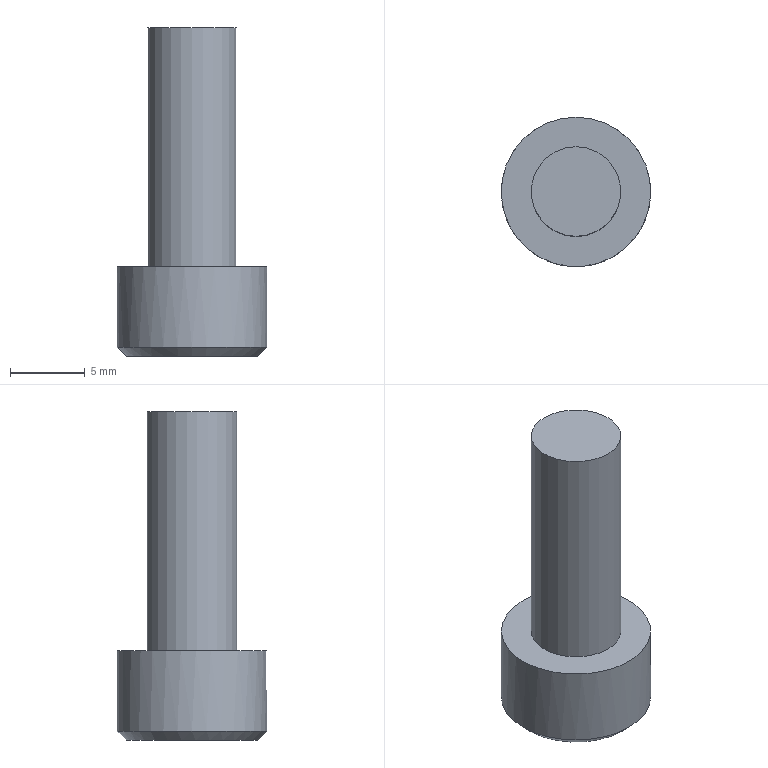Part | NX | features 5003_321_CB6-16 2 | 1 solid | 19 faces | box 10 x 10 x 22 mm | volume 843.416 mm3 | plane 15 | cylinder 2 | cone 2 | commonest cylinder face diameters 6 x1 10 x1
STEP:
#1=CARTESIAN_POINT('',(58.525,-211.4,-265.3));
#2=VERTEX_POINT('',#1);
#3=CARTESIAN_POINT('',(58.525,-207.,-265.3));
#4=DIRECTION('',(0.,0.,1.));
#5=DIRECTION('',(0.,-1.,0.));
#6=AXIS2_PLACEMENT_3D('',#3,#4,#5);
#7=CIRCLE('',#6,4.4);
#8=EDGE_CURVE('',#2,#2,#7,.F.);
#9=ORIENTED_EDGE('',*,*,#8,.T.);
#10=EDGE_LOOP('',(#9));
#11=FACE_BOUND('',#10,.T.);
#12=CARTESIAN_POINT('',(55.638,-207.,-265.3));
#13=VERTEX_POINT('',#12);
#14=CARTESIAN_POINT('',(57.082,-204.5,-265.3));
#15=VERTEX_POINT('',#14);
#16=CARTESIAN_POINT('',(55.638,-207.,-265.3));
#17=DIRECTION('',(0.5,0.866,0.));
#18=VECTOR('',#17,1000.);
#19=LINE('',#16,#18);
#20=EDGE_CURVE('',#13,#15,#19,.T.);
#21=ORIENTED_EDGE('',*,*,#20,.F.);
#22=CARTESIAN_POINT('',(57.082,-209.5,-265.3));
#23=VERTEX_POINT('',#22);
#24=CARTESIAN_POINT('',(57.082,-209.5,-265.3));
#25=DIRECTION('',(-0.5,0.866,0.));
#26=VECTOR('',#25,1000.);
#27=LINE('',#24,#26);
#28=EDGE_CURVE('',#23,#13,#27,.T.);
#29=ORIENTED_EDGE('',*,*,#28,.F.);
#30=CARTESIAN_POINT('',(59.968,-209.5,-265.3));
#31=VERTEX_POINT('',#30);
#32=CARTESIAN_POINT('',(59.968,-209.5,-265.3));
#33=DIRECTION('',(-1.,0.,0.));
#34=VECTOR('',#33,1000.);
#35=LINE('',#32,#34);
#36=EDGE_CURVE('',#31,#23,#35,.T.);
#37=ORIENTED_EDGE('',*,*,#36,.F.);
#38=CARTESIAN_POINT('',(61.412,-207.,-265.3));
#39=VERTEX_POINT('',#38);
#40=CARTESIAN_POINT('',(61.412,-207.,-265.3));
#41=DIRECTION('',(-0.5,-0.866,0.));
#42=VECTOR('',#41,1000.);
#43=LINE('',#40,#42);
#44=EDGE_CURVE('',#39,#31,#43,.T.);
#45=ORIENTED_EDGE('',*,*,#44,.F.);
#46=CARTESIAN_POINT('',(59.968,-204.5,-265.3));
#47=VERTEX_POINT('',#46);
#48=CARTESIAN_POINT('',(59.968,-204.5,-265.3));
#49=DIRECTION('',(0.5,-0.866,0.));
#50=VECTOR('',#49,1000.);
#51=LINE('',#48,#50);
#52=EDGE_CURVE('',#47,#39,#51,.T.);
#53=ORIENTED_EDGE('',*,*,#52,.F.);
#54=CARTESIAN_POINT('',(57.082,-204.5,-265.3));
#55=DIRECTION('',(1.,0.,0.));
#56=VECTOR('',#55,1000.);
#57=LINE('',#54,#56);
#58=EDGE_CURVE('',#15,#47,#57,.T.);
#59=ORIENTED_EDGE('',*,*,#58,.F.);
#60=EDGE_LOOP('',(#21,#29,#37,#45,#53,#59));
#61=FACE_BOUND('',#60,.T.);
#62=CARTESIAN_POINT('',(63.525,-207.,-265.3));
#63=DIRECTION('',(0.,0.,1.));
#64=DIRECTION('',(0.,-1.,0.));
#65=AXIS2_PLACEMENT_3D('',#62,#63,#64);
#66=PLANE('',#65);
#67=ADVANCED_FACE('',(#11,#61),#66,.F.);
#68=CARTESIAN_POINT('',(58.525,-204.,-243.3));
#69=VERTEX_POINT('',#68);
#70=CARTESIAN_POINT('',(58.525,-207.,-243.3));
#71=DIRECTION('',(0.,0.,-1.));
#72=DIRECTION('',(0.,1.,0.));
#73=AXIS2_PLACEMENT_3D('',#70,#71,#72);
#74=CIRCLE('',#73,3.);
#75=EDGE_CURVE('',#69,#69,#74,.T.);
#76=ORIENTED_EDGE('',*,*,#75,.F.);
#77=EDGE_LOOP('',(#76));
#78=FACE_BOUND('',#77,.T.);
#79=CARTESIAN_POINT('',(58.525,-207.,-243.3));
#80=DIRECTION('',(0.,0.,-1.));
#81=DIRECTION('',(0.,1.,0.));
#82=AXIS2_PLACEMENT_3D('',#79,#80,#81);
#83=PLANE('',#82);
#84=ADVANCED_FACE('',(#78),#83,.F.);
#85=CARTESIAN_POINT('',(58.525,-204.,-259.3));
#86=VERTEX_POINT('',#85);
#87=CARTESIAN_POINT('',(58.525,-207.,-259.3));
#88=DIRECTION('',(0.,0.,-1.));
#89=DIRECTION('',(0.,1.,0.));
#90=AXIS2_PLACEMENT_3D('',#87,#88,#89);
#91=CIRCLE('',#90,3.);
#92=EDGE_CURVE('',#86,#86,#91,.T.);
#93=ORIENTED_EDGE('',*,*,#92,.F.);
#94=EDGE_LOOP('',(#93));
#95=FACE_BOUND('',#94,.T.);
#96=ORIENTED_EDGE('',*,*,#75,.T.);
#97=EDGE_LOOP('',(#96));
#98=FACE_BOUND('',#97,.T.);
#99=CARTESIAN_POINT('',(58.525,-207.,-265.3));
#100=DIRECTION('',(0.,0.,-1.));
#101=DIRECTION('',(0.,1.,0.));
#102=AXIS2_PLACEMENT_3D('',#99,#100,#101);
#103=CYLINDRICAL_SURFACE('',#102,3.);
#104=ADVANCED_FACE('',(#95,#98),#103,.T.);
#105=CARTESIAN_POINT('',(58.525,-202.,-259.3));
#106=VERTEX_POINT('',#105);
#107=CARTESIAN_POINT('',(58.525,-207.,-259.3));
#108=DIRECTION('',(0.,0.,-1.));
#109=DIRECTION('',(0.,1.,0.));
#110=AXIS2_PLACEMENT_3D('',#107,#108,#109);
#111=CIRCLE('',#110,5.);
#112=EDGE_CURVE('',#106,#106,#111,.T.);
#113=ORIENTED_EDGE('',*,*,#112,.F.);
#114=EDGE_LOOP('',(#113));
#115=FACE_BOUND('',#114,.T.);
#116=ORIENTED_EDGE('',*,*,#92,.T.);
#117=EDGE_LOOP('',(#116));
#118=FACE_BOUND('',#117,.T.);
#119=CARTESIAN_POINT('',(61.525,-207.,-259.3));
#120=DIRECTION('',(0.,0.,-1.));
#121=DIRECTION('',(0.,1.,0.));
#122=AXIS2_PLACEMENT_3D('',#119,#120,#121);
#123=PLANE('',#122);
#124=ADVANCED_FACE('',(#115,#118),#123,.F.);
#125=CARTESIAN_POINT('',(58.525,-212.,-264.7));
#126=VERTEX_POINT('',#125);
#127=CARTESIAN_POINT('',(58.525,-207.,-264.7));
#128=DIRECTION('',(0.,0.,1.));
#129=DIRECTION('',(0.,-1.,0.));
#130=AXIS2_PLACEMENT_3D('',#127,#128,#129);
#131=CIRCLE('',#130,5.);
#132=EDGE_CURVE('',#126,#126,#131,.T.);
#133=ORIENTED_EDGE('',*,*,#132,.T.);
#134=EDGE_LOOP('',(#133));
#135=FACE_BOUND('',#134,.T.);
#136=ORIENTED_EDGE('',*,*,#112,.T.);
#137=EDGE_LOOP('',(#136));
#138=FACE_BOUND('',#137,.T.);
#139=CARTESIAN_POINT('',(58.525,-207.,-265.3));
#140=DIRECTION('',(0.,0.,-1.));
#141=DIRECTION('',(0.,1.,0.));
#142=AXIS2_PLACEMENT_3D('',#139,#140,#141);
#143=CYLINDRICAL_SURFACE('',#142,5.);
#144=ADVANCED_FACE('',(#135,#138),#143,.T.);
#145=ORIENTED_EDGE('',*,*,#132,.F.);
#146=EDGE_LOOP('',(#145));
#147=FACE_BOUND('',#146,.T.);
#148=ORIENTED_EDGE('',*,*,#8,.F.);
#149=EDGE_LOOP('',(#148));
#150=FACE_BOUND('',#149,.T.);
#151=CARTESIAN_POINT('',(58.525,-207.,-265.3));
#152=DIRECTION('',(0.,0.,1.));
#153=DIRECTION('',(0.,-1.,0.));
#154=AXIS2_PLACEMENT_3D('',#151,#152,#153);
#155=CONICAL_SURFACE('',#154,4.4,0.7854);
#156=ADVANCED_FACE('',(#147,#150),#155,.T.);
#157=CARTESIAN_POINT('',(57.082,-209.5,-262.3));
#158=VERTEX_POINT('',#157);
#159=CARTESIAN_POINT('',(56.36,-208.25,-262.3));
#160=VERTEX_POINT('',#159);
#161=CARTESIAN_POINT('',(57.082,-209.5,-262.3));
#162=DIRECTION('',(-0.5,0.866,0.));
#163=VECTOR('',#162,1000.);
#164=LINE('',#161,#163);
#165=EDGE_CURVE('',#158,#160,#164,.T.);
#166=ORIENTED_EDGE('',*,*,#165,.F.);
#167=CARTESIAN_POINT('',(57.082,-209.5,-262.3));
#168=DIRECTION('',(0.,0.,-1.));
#169=VECTOR('',#168,1000.);
#170=LINE('',#167,#169);
#171=EDGE_CURVE('',#158,#23,#170,.T.);
#172=ORIENTED_EDGE('',*,*,#171,.T.);
#173=ORIENTED_EDGE('',*,*,#28,.T.);
#174=CARTESIAN_POINT('',(55.638,-207.,-262.3));
#175=VERTEX_POINT('',#174);
#176=CARTESIAN_POINT('',(55.638,-207.,-262.3));
#177=DIRECTION('',(0.,0.,-1.));
#178=VECTOR('',#177,1000.);
#179=LINE('',#176,#178);
#180=EDGE_CURVE('',#175,#13,#179,.T.);
#181=ORIENTED_EDGE('',*,*,#180,.F.);
#182=CARTESIAN_POINT('',(57.082,-209.5,-262.3));
#183=DIRECTION('',(-0.5,0.866,0.));
#184=VECTOR('',#183,1000.);
#185=LINE('',#182,#184);
#186=EDGE_CURVE('',#160,#175,#185,.T.);
#187=ORIENTED_EDGE('',*,*,#186,.F.);
#188=EDGE_LOOP('',(#166,#172,#173,#181,#187));
#189=FACE_BOUND('',#188,.T.);
#190=CARTESIAN_POINT('',(57.082,-209.5,-262.3));
#191=DIRECTION('',(-0.866,-0.5,0.));
#192=DIRECTION('',(0.5,-0.866,0.));
#193=AXIS2_PLACEMENT_3D('',#190,#191,#192);
#194=PLANE('',#193);
#195=ADVANCED_FACE('',(#189),#194,.F.);
#196=CARTESIAN_POINT('',(59.968,-209.5,-262.3));
#197=VERTEX_POINT('',#196);
#198=CARTESIAN_POINT('',(58.525,-209.5,-262.3));
#199=VERTEX_POINT('',#198);
#200=CARTESIAN_POINT('',(59.968,-209.5,-262.3));
#201=DIRECTION('',(-1.,0.,0.));
#202=VECTOR('',#201,1000.);
#203=LINE('',#200,#202);
#204=EDGE_CURVE('',#197,#199,#203,.T.);
#205=ORIENTED_EDGE('',*,*,#204,.F.);
#206=CARTESIAN_POINT('',(59.968,-209.5,-262.3));
#207=DIRECTION('',(0.,0.,-1.));
#208=VECTOR('',#207,1000.);
#209=LINE('',#206,#208);
#210=EDGE_CURVE('',#197,#31,#209,.T.);
#211=ORIENTED_EDGE('',*,*,#210,.T.);
#212=ORIENTED_EDGE('',*,*,#36,.T.);
#213=ORIENTED_EDGE('',*,*,#171,.F.);
#214=CARTESIAN_POINT('',(59.968,-209.5,-262.3));
#215=DIRECTION('',(-1.,0.,0.));
#216=VECTOR('',#215,1000.);
#217=LINE('',#214,#216);
#218=EDGE_CURVE('',#199,#158,#217,.T.);
#219=ORIENTED_EDGE('',*,*,#218,.F.);
#220=EDGE_LOOP('',(#205,#211,#212,#213,#219));
#221=FACE_BOUND('',#220,.T.);
#222=CARTESIAN_POINT('',(59.968,-209.5,-262.3));
#223=DIRECTION('',(0.,-1.,0.));
#224=DIRECTION('',(1.,0.,0.));
#225=AXIS2_PLACEMENT_3D('',#222,#223,#224);
#226=PLANE('',#225);
#227=ADVANCED_FACE('',(#221),#226,.F.);
#228=CARTESIAN_POINT('',(61.412,-207.,-262.3));
#229=VERTEX_POINT('',#228);
#230=CARTESIAN_POINT('',(60.69,-208.25,-262.3));
#231=VERTEX_POINT('',#230);
#232=CARTESIAN_POINT('',(61.412,-207.,-262.3));
#233=DIRECTION('',(-0.5,-0.866,0.));
#234=VECTOR('',#233,1000.);
#235=LINE('',#232,#234);
#236=EDGE_CURVE('',#229,#231,#235,.T.);
#237=ORIENTED_EDGE('',*,*,#236,.F.);
#238=CARTESIAN_POINT('',(61.412,-207.,-262.3));
#239=DIRECTION('',(0.,0.,-1.));
#240=VECTOR('',#239,1000.);
#241=LINE('',#238,#240);
#242=EDGE_CURVE('',#229,#39,#241,.T.);
#243=ORIENTED_EDGE('',*,*,#242,.T.);
#244=ORIENTED_EDGE('',*,*,#44,.T.);
#245=ORIENTED_EDGE('',*,*,#210,.F.);
#246=CARTESIAN_POINT('',(61.412,-207.,-262.3));
#247=DIRECTION('',(-0.5,-0.866,0.));
#248=VECTOR('',#247,1000.);
#249=LINE('',#246,#248);
#250=EDGE_CURVE('',#231,#197,#249,.T.);
#251=ORIENTED_EDGE('',*,*,#250,.F.);
#252=EDGE_LOOP('',(#237,#243,#244,#245,#251));
#253=FACE_BOUND('',#252,.T.);
#254=CARTESIAN_POINT('',(61.412,-207.,-262.3));
#255=DIRECTION('',(0.866,-0.5,0.));
#256=DIRECTION('',(0.5,0.866,0.));
#257=AXIS2_PLACEMENT_3D('',#254,#255,#256);
#258=PLANE('',#257);
#259=ADVANCED_FACE('',(#253),#258,.F.);
#260=CARTESIAN_POINT('',(59.968,-204.5,-262.3));
#261=VERTEX_POINT('',#260);
#262=CARTESIAN_POINT('',(60.69,-205.75,-262.3));
#263=VERTEX_POINT('',#262);
#264=CARTESIAN_POINT('',(59.968,-204.5,-262.3));
#265=DIRECTION('',(0.5,-0.866,0.));
#266=VECTOR('',#265,1000.);
#267=LINE('',#264,#266);
#268=EDGE_CURVE('',#261,#263,#267,.T.);
#269=ORIENTED_EDGE('',*,*,#268,.F.);
#270=CARTESIAN_POINT('',(59.968,-204.5,-262.3));
#271=DIRECTION('',(0.,0.,-1.));
#272=VECTOR('',#271,1000.);
#273=LINE('',#270,#272);
#274=EDGE_CURVE('',#261,#47,#273,.T.);
#275=ORIENTED_EDGE('',*,*,#274,.T.);
#276=ORIENTED_EDGE('',*,*,#52,.T.);
#277=ORIENTED_EDGE('',*,*,#242,.F.);
#278=CARTESIAN_POINT('',(59.968,-204.5,-262.3));
#279=DIRECTION('',(0.5,-0.866,0.));
#280=VECTOR('',#279,1000.);
#281=LINE('',#278,#280);
#282=EDGE_CURVE('',#263,#229,#281,.T.);
#283=ORIENTED_EDGE('',*,*,#282,.F.);
#284=EDGE_LOOP('',(#269,#275,#276,#277,#283));
#285=FACE_BOUND('',#284,.T.);
#286=CARTESIAN_POINT('',(59.968,-204.5,-262.3));
#287=DIRECTION('',(0.866,0.5,0.));
#288=DIRECTION('',(-0.5,0.866,0.));
#289=AXIS2_PLACEMENT_3D('',#286,#287,#288);
#290=PLANE('',#289);
#291=ADVANCED_FACE('',(#285),#290,.F.);
#292=CARTESIAN_POINT('',(57.082,-204.5,-262.3));
#293=VERTEX_POINT('',#292);
#294=CARTESIAN_POINT('',(58.525,-204.5,-262.3));
#295=VERTEX_POINT('',#294);
#296=CARTESIAN_POINT('',(57.082,-204.5,-262.3));
#297=DIRECTION('',(1.,0.,0.));
#298=VECTOR('',#297,1000.);
#299=LINE('',#296,#298);
#300=EDGE_CURVE('',#293,#295,#299,.T.);
#301=ORIENTED_EDGE('',*,*,#300,.F.);
#302=CARTESIAN_POINT('',(57.082,-204.5,-262.3));
#303=DIRECTION('',(0.,0.,-1.));
#304=VECTOR('',#303,1000.);
#305=LINE('',#302,#304);
#306=EDGE_CURVE('',#293,#15,#305,.T.);
#307=ORIENTED_EDGE('',*,*,#306,.T.);
#308=ORIENTED_EDGE('',*,*,#58,.T.);
#309=ORIENTED_EDGE('',*,*,#274,.F.);
#310=CARTESIAN_POINT('',(57.082,-204.5,-262.3));
#311=DIRECTION('',(1.,0.,0.));
#312=VECTOR('',#311,1000.);
#313=LINE('',#310,#312);
#314=EDGE_CURVE('',#295,#261,#313,.T.);
#315=ORIENTED_EDGE('',*,*,#314,.F.);
#316=EDGE_LOOP('',(#301,#307,#308,#309,#315));
#317=FACE_BOUND('',#316,.T.);
#318=CARTESIAN_POINT('',(57.082,-204.5,-262.3));
#319=DIRECTION('',(0.,1.,0.));
#320=DIRECTION('',(0.,0.,1.));
#321=AXIS2_PLACEMENT_3D('',#318,#319,#320);
#322=PLANE('',#321);
#323=ADVANCED_FACE('',(#317),#322,.F.);
#324=CARTESIAN_POINT('',(56.36,-205.75,-262.3));
#325=VERTEX_POINT('',#324);
#326=CARTESIAN_POINT('',(55.638,-207.,-262.3));
#327=DIRECTION('',(0.5,0.866,0.));
#328=VECTOR('',#327,1000.);
#329=LINE('',#326,#328);
#330=EDGE_CURVE('',#175,#325,#329,.T.);
#331=ORIENTED_EDGE('',*,*,#330,.F.);
#332=ORIENTED_EDGE('',*,*,#180,.T.);
#333=ORIENTED_EDGE('',*,*,#20,.T.);
#334=ORIENTED_EDGE('',*,*,#306,.F.);
#335=CARTESIAN_POINT('',(55.638,-207.,-262.3));
#336=DIRECTION('',(0.5,0.866,0.));
#337=VECTOR('',#336,1000.);
#338=LINE('',#335,#337);
#339=EDGE_CURVE('',#325,#293,#338,.T.);
#340=ORIENTED_EDGE('',*,*,#339,.F.);
#341=EDGE_LOOP('',(#331,#332,#333,#334,#340));
#342=FACE_BOUND('',#341,.T.);
#343=CARTESIAN_POINT('',(55.638,-207.,-262.3));
#344=DIRECTION('',(-0.866,0.5,0.));
#345=DIRECTION('',(-0.5,-0.866,0.));
#346=AXIS2_PLACEMENT_3D('',#343,#344,#345);
#347=PLANE('',#346);
#348=ADVANCED_FACE('',(#342),#347,.F.);
#349=ORIENTED_EDGE('',*,*,#314,.T.);
#350=ORIENTED_EDGE('',*,*,#268,.T.);
#351=CARTESIAN_POINT('',(58.525,-207.,-262.3));
#352=DIRECTION('',(0.,0.,-1.));
#353=DIRECTION('',(-1.,0.,0.));
#354=AXIS2_PLACEMENT_3D('',#351,#352,#353);
#355=CIRCLE('',#354,2.5);
#356=EDGE_CURVE('',#295,#263,#355,.T.);
#357=ORIENTED_EDGE('',*,*,#356,.F.);
#358=EDGE_LOOP('',(#349,#350,#357));
#359=FACE_BOUND('',#358,.T.);
#360=CARTESIAN_POINT('',(58.525,-207.,-262.3));
#361=DIRECTION('',(0.,0.,-1.));
#362=DIRECTION('',(0.,1.,0.));
#363=AXIS2_PLACEMENT_3D('',#360,#361,#362);
#364=PLANE('',#363);
#365=ADVANCED_FACE('',(#359),#364,.T.);
#366=ORIENTED_EDGE('',*,*,#282,.T.);
#367=ORIENTED_EDGE('',*,*,#236,.T.);
#368=CARTESIAN_POINT('',(58.525,-207.,-262.3));
#369=DIRECTION('',(0.,0.,-1.));
#370=DIRECTION('',(-1.,0.,0.));
#371=AXIS2_PLACEMENT_3D('',#368,#369,#370);
#372=CIRCLE('',#371,2.5);
#373=EDGE_CURVE('',#263,#231,#372,.T.);
#374=ORIENTED_EDGE('',*,*,#373,.F.);
#375=EDGE_LOOP('',(#366,#367,#374));
#376=FACE_BOUND('',#375,.T.);
#377=CARTESIAN_POINT('',(58.525,-207.,-262.3));
#378=DIRECTION('',(0.,0.,-1.));
#379=DIRECTION('',(0.,1.,0.));
#380=AXIS2_PLACEMENT_3D('',#377,#378,#379);
#381=PLANE('',#380);
#382=ADVANCED_FACE('',(#376),#381,.T.);
#383=ORIENTED_EDGE('',*,*,#250,.T.);
#384=ORIENTED_EDGE('',*,*,#204,.T.);
#385=CARTESIAN_POINT('',(58.525,-207.,-262.3));
#386=DIRECTION('',(0.,0.,-1.));
#387=DIRECTION('',(-1.,0.,0.));
#388=AXIS2_PLACEMENT_3D('',#385,#386,#387);
#389=CIRCLE('',#388,2.5);
#390=EDGE_CURVE('',#231,#199,#389,.T.);
#391=ORIENTED_EDGE('',*,*,#390,.F.);
#392=EDGE_LOOP('',(#383,#384,#391));
#393=FACE_BOUND('',#392,.T.);
#394=CARTESIAN_POINT('',(58.525,-207.,-262.3));
#395=DIRECTION('',(0.,0.,-1.));
#396=DIRECTION('',(0.,1.,0.));
#397=AXIS2_PLACEMENT_3D('',#394,#395,#396);
#398=PLANE('',#397);
#399=ADVANCED_FACE('',(#393),#398,.T.);
#400=ORIENTED_EDGE('',*,*,#218,.T.);
#401=ORIENTED_EDGE('',*,*,#165,.T.);
#402=CARTESIAN_POINT('',(58.525,-207.,-262.3));
#403=DIRECTION('',(0.,0.,-1.));
#404=DIRECTION('',(-1.,0.,0.));
#405=AXIS2_PLACEMENT_3D('',#402,#403,#404);
#406=CIRCLE('',#405,2.5);
#407=EDGE_CURVE('',#199,#160,#406,.T.);
#408=ORIENTED_EDGE('',*,*,#407,.F.);
#409=EDGE_LOOP('',(#400,#401,#408));
#410=FACE_BOUND('',#409,.T.);
#411=CARTESIAN_POINT('',(58.525,-207.,-262.3));
#412=DIRECTION('',(0.,0.,-1.));
#413=DIRECTION('',(0.,1.,0.));
#414=AXIS2_PLACEMENT_3D('',#411,#412,#413);
#415=PLANE('',#414);
#416=ADVANCED_FACE('',(#410),#415,.T.);
#417=ORIENTED_EDGE('',*,*,#186,.T.);
#418=ORIENTED_EDGE('',*,*,#330,.T.);
#419=CARTESIAN_POINT('',(58.525,-207.,-262.3));
#420=DIRECTION('',(0.,0.,-1.));
#421=DIRECTION('',(-1.,0.,0.));
#422=AXIS2_PLACEMENT_3D('',#419,#420,#421);
#423=CIRCLE('',#422,2.5);
#424=EDGE_CURVE('',#160,#325,#423,.T.);
#425=ORIENTED_EDGE('',*,*,#424,.F.);
#426=EDGE_LOOP('',(#417,#418,#425));
#427=FACE_BOUND('',#426,.T.);
#428=CARTESIAN_POINT('',(58.525,-207.,-262.3));
#429=DIRECTION('',(0.,0.,-1.));
#430=DIRECTION('',(0.,1.,0.));
#431=AXIS2_PLACEMENT_3D('',#428,#429,#430);
#432=PLANE('',#431);
#433=ADVANCED_FACE('',(#427),#432,.T.);
#434=ORIENTED_EDGE('',*,*,#339,.T.);
#435=ORIENTED_EDGE('',*,*,#300,.T.);
#436=CARTESIAN_POINT('',(58.525,-207.,-262.3));
#437=DIRECTION('',(0.,0.,-1.));
#438=DIRECTION('',(-1.,0.,0.));
#439=AXIS2_PLACEMENT_3D('',#436,#437,#438);
#440=CIRCLE('',#439,2.5);
#441=EDGE_CURVE('',#325,#295,#440,.T.);
#442=ORIENTED_EDGE('',*,*,#441,.F.);
#443=EDGE_LOOP('',(#434,#435,#442));
#444=FACE_BOUND('',#443,.T.);
#445=CARTESIAN_POINT('',(58.525,-207.,-262.3));
#446=DIRECTION('',(0.,0.,-1.));
#447=DIRECTION('',(0.,1.,0.));
#448=AXIS2_PLACEMENT_3D('',#445,#446,#447);
#449=PLANE('',#448);
#450=ADVANCED_FACE('',(#444),#449,.T.);
#451=ORIENTED_EDGE('',*,*,#441,.T.);
#452=ORIENTED_EDGE('',*,*,#356,.T.);
#453=ORIENTED_EDGE('',*,*,#373,.T.);
#454=ORIENTED_EDGE('',*,*,#390,.T.);
#455=ORIENTED_EDGE('',*,*,#407,.T.);
#456=ORIENTED_EDGE('',*,*,#424,.T.);
#457=EDGE_LOOP('',(#451,#452,#453,#454,#455,#456));
#458=FACE_BOUND('',#457,.T.);
#459=CARTESIAN_POINT('',(58.525,-207.,-260.798));
#460=VERTEX_POINT('',#459);
#461=VERTEX_LOOP('',#460);
#462=FACE_BOUND('',#461,.T.);
#463=CARTESIAN_POINT('',(58.525,-207.,-260.798));
#464=DIRECTION('',(0.,0.,-1.));
#465=DIRECTION('',(-1.,0.,0.));
#466=AXIS2_PLACEMENT_3D('',#463,#464,#465);
#467=CONICAL_SURFACE('',#466,0.,1.03);
#468=ADVANCED_FACE('',(#458,#462),#467,.F.);
#469=CLOSED_SHELL('',(#67,#84,#104,#124,#144,#156,#195,#227,#259,#291,#323,#348,#365,#382,#399,#416,#433,#450,#468));
#470=MANIFOLD_SOLID_BREP('',#469);
#471=(LENGTH_UNIT()NAMED_UNIT(*)SI_UNIT(.MILLI.,.METRE.));
#472=UNCERTAINTY_MEASURE_WITH_UNIT(LENGTH_MEASURE(0.00001),#471,'','');
#473=(NAMED_UNIT(*)PLANE_ANGLE_UNIT()SI_UNIT($,.RADIAN.));
#474=(NAMED_UNIT(*)SI_UNIT($,.STERADIAN.)SOLID_ANGLE_UNIT());
#475=(GEOMETRIC_REPRESENTATION_CONTEXT(3)GLOBAL_UNCERTAINTY_ASSIGNED_CONTEXT((#472))GLOBAL_UNIT_ASSIGNED_CONTEXT((#471,#473,#474))REPRESENTATION_CONTEXT('',''));
#476=ADVANCED_BREP_SHAPE_REPRESENTATION('',(#470),#475);